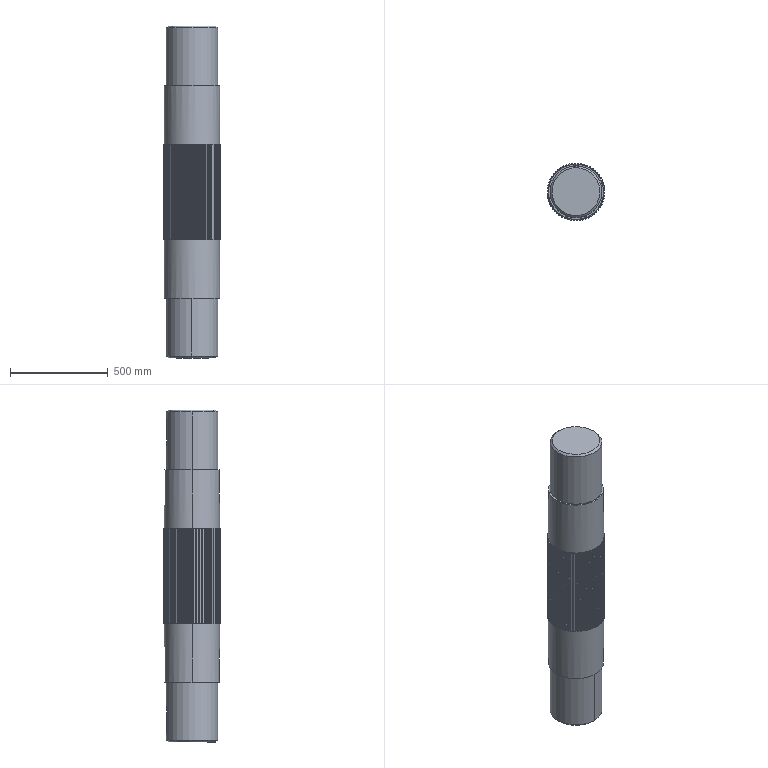Part | SolidWorks | features ICE 7, 3DProfileFeature 1, Chamfer 1, CirPattern 1, Extrusion 1, Fillet 1 | 1 solid | 450 faces | box 294.723 x 294.709 x 1700 mm | volume 103257734 mm3 | cylinder 202 | plane 124 | spline 120 | cone 4 | commonest cylinder face diameters 4 x136 295 x58 265 x6 282.5 x2